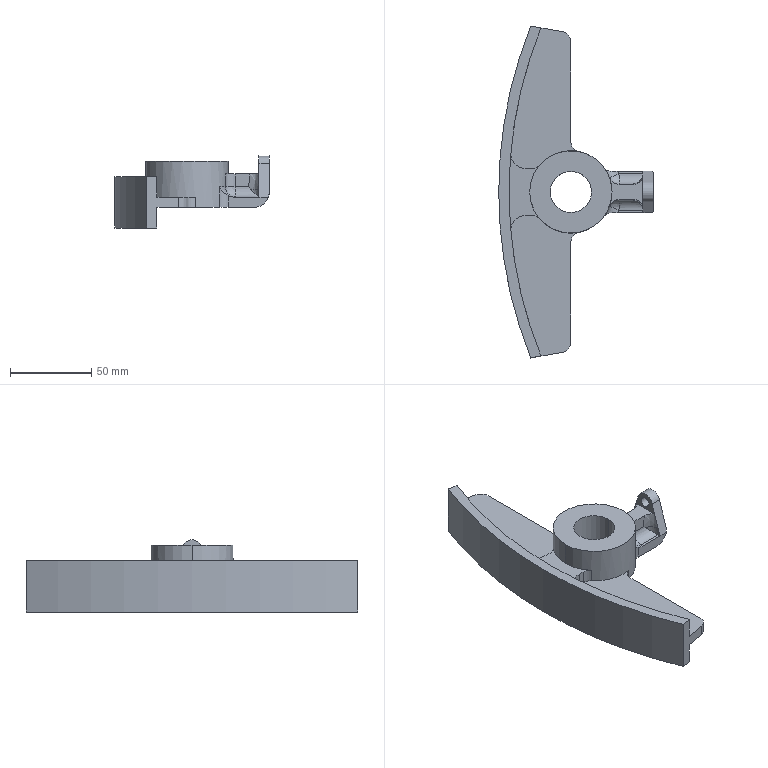Part | SolidWorks | features Fillet 7, ICE 6, Extrusion 1, Rib 1 | 1 solid | 59 faces | box 95.24 x 204.62 x 44.45 mm | volume 132567 mm3 | cylinder 27 | plane 26 | spline 2 | sphere 2 | torus 2 | commonest cylinder face diameters 12.7 x15 6.35 x2 19.06 x2 25.43 x2 50.8 x2 540 x2